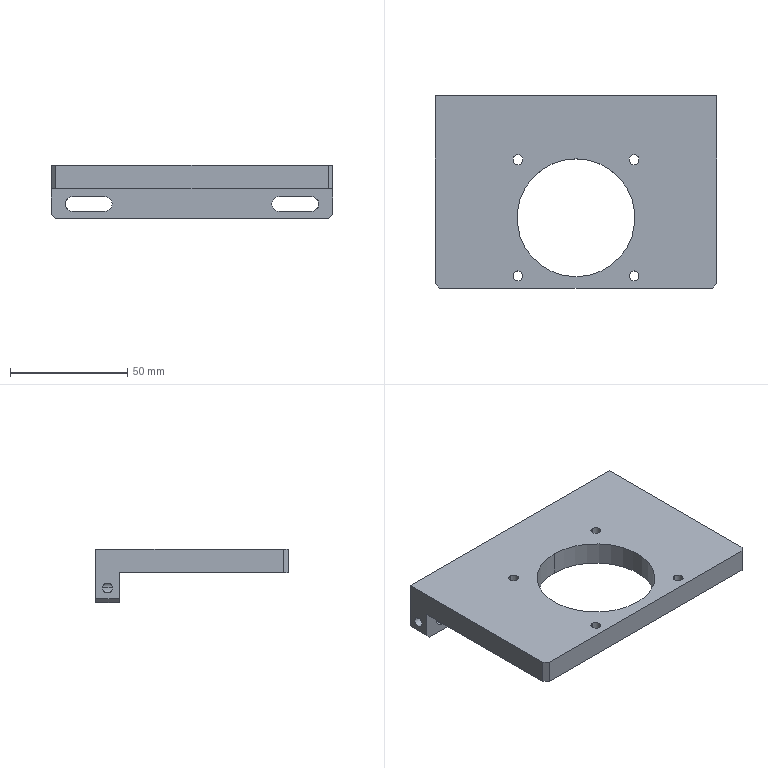NC program | NX | posted with a generic post | part box 120 x 82 x 22.8 mm
Lines 1 to 877 of 2242:
N10 G17 G21 G94 G90
(ZLEVEL_PROFILE_COPY_1 , TOOL : D4)
N12 T11 M6
N14 G54
N16 G17 G0 G90 X-42.486 Y6.25 B0. C0. S9500 M3
N18 G43 Z30. H11
N20 Z1.5
N22 G94 G1 X-51.114 Z1.048 F1000.
N24 X-51.591 Y6.018 Z1.02
N26 X-51.919 Y5.6 Z0.992
N28 X-52.03 Y5.084 Z0.964
N30 X-51.909 Y4.579 Z0.937
N32 X-51.582 Y4.175 Z0.91
N34 X-51.114 Y3.95 Z0.883
N36 X-36.886 Z0.137
N38 X-36.305 Y4.277 Z0.102
N40 X-35.993 Y4.866 Z0.067
N42 X-36.007 Y5.394 Z0.04
N44 X-36.327 Y5.945 Z0.006
N46 X-36.886 Y6.25 Z-0.027
N48 X-44. Z-0.4
N50 X-50.85 F1500.
N52 G3 X-52. Y5.1 R1.15
N54 X-50.85 Y3.95 R1.15
N56 G1 X-37.15
N58 G3 X-36. Y5.1 R1.15
N60 X-37.15 Y6.25 R1.15
N62 G1 X-44.
N64 X-45.713 Z-0.42
N66 X-47.425 Z-0.44
N68 X-49.138 Z-0.459
N70 X-50.85 Y6.233 Z-0.479
N72 X-51.18 Y6.18 Z-0.483
N74 X-51.343 Y6.112 Z-0.485
N76 X-51.518 Y6.004 Z-0.488
N78 X-51.652 Y5.902 Z-0.49
N80 X-51.734 Y5.793 Z-0.491
N82 X-51.906 Y5.487 Z-0.495
N84 X-51.952 Y5.337 Z-0.497
N86 X-51.976 Y5.035 Z-0.501
N88 X-51.95 Y4.838 Z-0.503
N90 X-51.85 Y4.575 Z-0.506
N92 X-51.726 Y4.393 Z-0.509
N94 X-51.513 Y4.191 Z-0.512
N96 X-51.335 Y4.084 Z-0.515
N98 X-51.2 Y4.028 Z-0.517
N100 X-51.131 Y4.003
N102 X-51.037 Y3.99 Z-0.519
N104 X-50.85 Y3.967 Z-0.521
N106 X-49.138 Y3.95 Z-0.541
N108 X-38.863 Z-0.659
N110 X-37.15 Y3.967 Z-0.679
N112 X-36.869 Y4.002 Z-0.683
N114 X-36.713 Y4.065 Z-0.684
N116 X-36.447 Y4.222 Z-0.688
N118 X-36.338 Y4.309 Z-0.69
N120 X-36.197 Y4.496 Z-0.693
N122 X-36.102 Y4.69 Z-0.695
N124 X-36.035 Y4.953 Z-0.698
N126 X-36.019 Y5.13 Z-0.7
N128 X-36.049 Y5.357 Z-0.703
N130 X-36.119 Y5.551 Z-0.705
N132 X-36.26 Y5.788 Z-0.709
N134 X-36.359 Y5.912 Z-0.711
N136 X-36.534 Y6.043 Z-0.713
N138 X-36.727 Y6.141 Z-0.716
N140 X-36.914 Y6.204 Z-0.718
N142 X-37.15 Y6.233 Z-0.721
N144 X-38.863 Y6.25 Z-0.741
N146 X-40.575 Z-0.76
N148 X-42.288 Z-0.78
N150 X-44. Z-0.8
N152 X-45.713 Z-0.82
N154 X-47.425 Z-0.84
N156 X-49.138 Z-0.859
N158 X-50.85 Y6.233 Z-0.879
N160 X-51.18 Y6.18 Z-0.883
N162 X-51.343 Y6.112 Z-0.885
N164 X-51.518 Y6.004 Z-0.888
N166 X-51.652 Y5.902 Z-0.89
N168 X-51.734 Y5.793 Z-0.891
N170 X-51.906 Y5.487 Z-0.895
N172 X-51.952 Y5.337 Z-0.897
N174 X-51.976 Y5.035 Z-0.901
N176 X-51.95 Y4.838 Z-0.903
N178 X-51.85 Y4.575 Z-0.906
N180 X-51.726 Y4.393 Z-0.909
N182 X-51.513 Y4.191 Z-0.912
N184 X-51.335 Y4.084 Z-0.915
N186 X-51.2 Y4.028 Z-0.917
N188 X-51.131 Y4.003
N190 X-51.037 Y3.99 Z-0.919
N192 X-50.85 Y3.967 Z-0.921
N194 X-49.138 Y3.95 Z-0.941
N196 X-38.863 Z-1.059
N198 X-37.15 Y3.967 Z-1.079
N200 X-36.869 Y4.002 Z-1.083
N202 X-36.713 Y4.065 Z-1.084
N204 X-36.447 Y4.222 Z-1.088
N206 X-36.338 Y4.309 Z-1.09
N208 X-36.197 Y4.496 Z-1.093
N210 X-36.102 Y4.69 Z-1.095
N212 X-36.035 Y4.953 Z-1.098
N214 X-36.019 Y5.13 Z-1.1
N216 X-36.049 Y5.357 Z-1.103
N218 X-36.119 Y5.551 Z-1.105
N220 X-36.26 Y5.788 Z-1.109
N222 X-36.359 Y5.912 Z-1.111
N224 X-36.534 Y6.043 Z-1.113
N226 X-36.727 Y6.141 Z-1.116
N228 X-36.914 Y6.204 Z-1.118
N230 X-37.15 Y6.233 Z-1.121
N232 X-38.863 Y6.25 Z-1.141
N234 X-40.575 Z-1.16
N236 X-42.288 Z-1.18
N238 X-44. Z-1.2
N240 X-45.713 Z-1.22
N242 X-47.425 Z-1.24
N244 X-49.138 Z-1.259
N246 X-50.85 Y6.233 Z-1.279
N248 X-51.18 Y6.18 Z-1.283
N250 X-51.343 Y6.112 Z-1.285
N252 X-51.518 Y6.004 Z-1.288
N254 X-51.652 Y5.902 Z-1.29
N256 X-51.734 Y5.793 Z-1.291
N258 X-51.906 Y5.487 Z-1.295
N260 X-51.952 Y5.337 Z-1.297
N262 X-51.976 Y5.035 Z-1.301
N264 X-51.95 Y4.838 Z-1.303
N266 X-51.85 Y4.575 Z-1.306
N268 X-51.726 Y4.393 Z-1.309
N270 X-51.513 Y4.191 Z-1.312
N272 X-51.335 Y4.084 Z-1.315
N274 X-51.2 Y4.028 Z-1.317
N276 X-51.131 Y4.003
N278 X-51.037 Y3.99 Z-1.319
N280 X-50.85 Y3.967 Z-1.321
N282 X-49.138 Y3.95 Z-1.341
N284 X-38.863 Z-1.459
N286 X-37.15 Y3.967 Z-1.479
N288 X-36.869 Y4.002 Z-1.483
N290 X-36.713 Y4.065 Z-1.484
N292 X-36.447 Y4.222 Z-1.488
N294 X-36.338 Y4.309 Z-1.49
N296 X-36.197 Y4.496 Z-1.493
N298 X-36.102 Y4.69 Z-1.495
N300 X-36.035 Y4.953 Z-1.498
N302 X-36.019 Y5.13 Z-1.5
N304 X-36.049 Y5.357 Z-1.503
N306 X-36.119 Y5.551 Z-1.505
N308 X-36.26 Y5.788 Z-1.509
N310 X-36.359 Y5.912 Z-1.511
N312 X-36.534 Y6.043 Z-1.513
N314 X-36.727 Y6.141 Z-1.516
N316 X-36.914 Y6.204 Z-1.518
N318 X-37.15 Y6.233 Z-1.521
N320 X-38.863 Y6.25 Z-1.541
N322 X-40.575 Z-1.56
N324 X-42.288 Z-1.58
N326 X-44. Z-1.6
N328 X-45.713 Z-1.62
N330 X-47.425 Z-1.64
N332 X-49.138 Z-1.659
N334 X-50.85 Y6.233 Z-1.679
N336 X-51.18 Y6.18 Z-1.683
N338 X-51.343 Y6.112 Z-1.685
N340 X-51.518 Y6.004 Z-1.688
N342 X-51.652 Y5.902 Z-1.69
N344 X-51.734 Y5.793 Z-1.691
N346 X-51.906 Y5.487 Z-1.695
N348 X-51.952 Y5.337 Z-1.697
N350 X-51.976 Y5.035 Z-1.701
N352 X-51.95 Y4.838 Z-1.703
N354 X-51.85 Y4.575 Z-1.706
N356 X-51.726 Y4.393 Z-1.709
N358 X-51.513 Y4.191 Z-1.712
N360 X-51.335 Y4.084 Z-1.715
N362 X-51.2 Y4.028 Z-1.717
N364 X-51.131 Y4.003
N366 X-51.037 Y3.99 Z-1.719
N368 X-50.85 Y3.967 Z-1.721
N370 X-49.138 Y3.95 Z-1.741
N372 X-38.863 Z-1.859
N374 X-37.15 Y3.967 Z-1.879
N376 X-36.869 Y4.002 Z-1.883
N378 X-36.713 Y4.065 Z-1.884
N380 X-36.447 Y4.222 Z-1.888
N382 X-36.338 Y4.309 Z-1.89
N384 X-36.197 Y4.496 Z-1.893
N386 X-36.102 Y4.69 Z-1.895
N388 X-36.035 Y4.953 Z-1.898
N390 X-36.019 Y5.13 Z-1.9
N392 X-36.049 Y5.357 Z-1.903
N394 X-36.119 Y5.551 Z-1.905
N396 X-36.26 Y5.788 Z-1.909
N398 X-36.359 Y5.912 Z-1.911
N400 X-36.534 Y6.043 Z-1.913
N402 X-36.727 Y6.141 Z-1.916
N404 X-36.914 Y6.204 Z-1.918
N406 X-37.15 Y6.233 Z-1.921
N408 X-38.863 Y6.25 Z-1.941
N410 X-40.575 Z-1.96
N412 X-42.288 Z-1.98
N414 X-44. Z-2.
N416 X-45.713 Z-2.02
N418 X-47.425 Z-2.04
N420 X-49.138 Z-2.059
N422 X-50.85 Y6.233 Z-2.079
N424 X-51.18 Y6.18 Z-2.083
N426 X-51.343 Y6.112 Z-2.085
N428 X-51.518 Y6.004 Z-2.088
N430 X-51.652 Y5.902 Z-2.09
N432 X-51.734 Y5.793 Z-2.091
N434 X-51.906 Y5.487 Z-2.095
N436 X-51.952 Y5.337 Z-2.097
N438 X-51.976 Y5.035 Z-2.101
N440 X-51.95 Y4.838 Z-2.103
N442 X-51.85 Y4.575 Z-2.106
N444 X-51.726 Y4.393 Z-2.109
N446 X-51.513 Y4.191 Z-2.112
N448 X-51.335 Y4.084 Z-2.115
N450 X-51.2 Y4.028 Z-2.117
N452 X-51.131 Y4.003
N454 X-51.037 Y3.99 Z-2.119
N456 X-50.85 Y3.967 Z-2.121
N458 X-49.138 Y3.95 Z-2.141
N460 X-38.863 Z-2.259
N462 X-37.15 Y3.967 Z-2.279
N464 X-36.869 Y4.002 Z-2.283
N466 X-36.713 Y4.065 Z-2.284
N468 X-36.447 Y4.222 Z-2.288
N470 X-36.338 Y4.309 Z-2.29
N472 X-36.197 Y4.496 Z-2.293
N474 X-36.102 Y4.69 Z-2.295
N476 X-36.035 Y4.953 Z-2.298
N478 X-36.019 Y5.13 Z-2.3
N480 X-36.049 Y5.357 Z-2.303
N482 X-36.119 Y5.551 Z-2.305
N484 X-36.26 Y5.788 Z-2.309
N486 X-36.359 Y5.912 Z-2.311
N488 X-36.534 Y6.043 Z-2.313
N490 X-36.727 Y6.141 Z-2.316
N492 X-36.914 Y6.204 Z-2.318
N494 X-37.15 Y6.233 Z-2.321
N496 X-38.863 Y6.25 Z-2.341
N498 X-40.575 Z-2.36
N500 X-42.288 Z-2.38
N502 X-44. Z-2.4
N504 X-45.713 Z-2.42
N506 X-47.425 Z-2.44
N508 X-49.138 Z-2.459
N510 X-50.85 Y6.233 Z-2.479
N512 X-51.18 Y6.18 Z-2.483
N514 X-51.343 Y6.112 Z-2.485
N516 X-51.518 Y6.004 Z-2.488
N518 X-51.652 Y5.902 Z-2.49
N520 X-51.734 Y5.793 Z-2.491
N522 X-51.906 Y5.487 Z-2.495
N524 X-51.952 Y5.337 Z-2.497
N526 X-51.976 Y5.035 Z-2.501
N528 X-51.95 Y4.838 Z-2.503
N530 X-51.85 Y4.575 Z-2.506
N532 X-51.726 Y4.393 Z-2.509
N534 X-51.513 Y4.191 Z-2.512
N536 X-51.335 Y4.084 Z-2.515
N538 X-51.2 Y4.028 Z-2.517
N540 X-51.131 Y4.003
N542 X-51.037 Y3.99 Z-2.519
N544 X-50.85 Y3.967 Z-2.521
N546 X-49.138 Y3.95 Z-2.541
N548 X-38.863 Z-2.659
N550 X-37.15 Y3.967 Z-2.679
N552 X-36.869 Y4.002 Z-2.683
N554 X-36.713 Y4.065 Z-2.684
N556 X-36.447 Y4.222 Z-2.688
N558 X-36.338 Y4.309 Z-2.69
N560 X-36.197 Y4.496 Z-2.693
N562 X-36.102 Y4.69 Z-2.695
N564 X-36.035 Y4.953 Z-2.698
N566 X-36.019 Y5.13 Z-2.7
N568 X-36.049 Y5.357 Z-2.703
N570 X-36.119 Y5.551 Z-2.705
N572 X-36.26 Y5.788 Z-2.709
N574 X-36.359 Y5.912 Z-2.711
N576 X-36.534 Y6.043 Z-2.713
N578 X-36.727 Y6.141 Z-2.716
N580 X-36.914 Y6.204 Z-2.718
N582 X-37.15 Y6.233 Z-2.721
N584 X-38.863 Y6.25 Z-2.741
N586 X-40.575 Z-2.76
N588 X-42.288 Z-2.78
N590 X-44. Z-2.8
N592 X-45.713 Z-2.82
N594 X-47.425 Z-2.84
N596 X-49.138 Z-2.859
N598 X-50.85 Y6.233 Z-2.879
N600 X-51.18 Y6.18 Z-2.883
N602 X-51.343 Y6.112 Z-2.885
N604 X-51.518 Y6.004 Z-2.888
N606 X-51.652 Y5.902 Z-2.89
N608 X-51.734 Y5.793 Z-2.891
N610 X-51.906 Y5.487 Z-2.895
N612 X-51.952 Y5.337 Z-2.897
N614 X-51.976 Y5.035 Z-2.901
N616 X-51.95 Y4.838 Z-2.903
N618 X-51.85 Y4.575 Z-2.906
N620 X-51.726 Y4.393 Z-2.909
N622 X-51.513 Y4.191 Z-2.912
N624 X-51.335 Y4.084 Z-2.915
N626 X-51.2 Y4.028 Z-2.917
N628 X-51.131 Y4.003
N630 X-51.037 Y3.99 Z-2.919
N632 X-50.85 Y3.967 Z-2.921
N634 X-49.138 Y3.95 Z-2.941
N636 X-38.863 Z-3.059
N638 X-37.15 Y3.967 Z-3.079
N640 X-36.869 Y4.002 Z-3.083
N642 X-36.713 Y4.065 Z-3.084
N644 X-36.447 Y4.222 Z-3.088
N646 X-36.338 Y4.309 Z-3.09
N648 X-36.197 Y4.496 Z-3.093
N650 X-36.102 Y4.69 Z-3.095
N652 X-36.035 Y4.953 Z-3.098
N654 X-36.019 Y5.13 Z-3.1
N656 X-36.049 Y5.357 Z-3.103
N658 X-36.119 Y5.551 Z-3.105
N660 X-36.26 Y5.788 Z-3.109
N662 X-36.359 Y5.912 Z-3.111
N664 X-36.534 Y6.043 Z-3.113
N666 X-36.727 Y6.141 Z-3.116
N668 X-36.914 Y6.204 Z-3.118
N670 X-37.15 Y6.233 Z-3.121
N672 X-38.863 Y6.25 Z-3.141
N674 X-40.575 Z-3.16
N676 X-42.288 Z-3.18
N678 X-44. Z-3.2
N680 X-45.713 Z-3.22
N682 X-47.425 Z-3.24
N684 X-49.138 Z-3.259
N686 X-50.85 Y6.233 Z-3.279
N688 X-51.18 Y6.18 Z-3.283
N690 X-51.343 Y6.112 Z-3.285
N692 X-51.518 Y6.004 Z-3.288
N694 X-51.652 Y5.902 Z-3.29
N696 X-51.734 Y5.793 Z-3.291
N698 X-51.906 Y5.487 Z-3.295
N700 X-51.952 Y5.337 Z-3.297
N702 X-51.976 Y5.035 Z-3.301
N704 X-51.95 Y4.838 Z-3.303
N706 X-51.85 Y4.575 Z-3.306
N708 X-51.726 Y4.393 Z-3.309
N710 X-51.513 Y4.191 Z-3.312
N712 X-51.335 Y4.084 Z-3.315
N714 X-51.2 Y4.028 Z-3.317
N716 X-51.131 Y4.003
N718 X-51.037 Y3.99 Z-3.319
N720 X-50.85 Y3.967 Z-3.321
N722 X-49.138 Y3.95 Z-3.341
N724 X-38.863 Z-3.459
N726 X-37.15 Y3.967 Z-3.479
N728 X-36.869 Y4.002 Z-3.483
N730 X-36.713 Y4.065 Z-3.484
N732 X-36.447 Y4.222 Z-3.488
N734 X-36.338 Y4.309 Z-3.49
N736 X-36.197 Y4.496 Z-3.493
N738 X-36.102 Y4.69 Z-3.495
N740 X-36.035 Y4.953 Z-3.498
N742 X-36.019 Y5.13 Z-3.5
N744 X-36.049 Y5.357 Z-3.503
N746 X-36.119 Y5.551 Z-3.505
N748 X-36.26 Y5.788 Z-3.509
N750 X-36.359 Y5.912 Z-3.511
N752 X-36.534 Y6.043 Z-3.513
N754 X-36.727 Y6.141 Z-3.516
N756 X-36.914 Y6.204 Z-3.518
N758 X-37.15 Y6.233 Z-3.521
N760 X-38.863 Y6.25 Z-3.541
N762 X-40.575 Z-3.56
N764 X-42.288 Z-3.58
N766 X-44. Z-3.6
N768 X-45.713 Z-3.62
N770 X-47.425 Z-3.64
N772 X-49.138 Z-3.659
N774 X-50.85 Y6.233 Z-3.679
N776 X-51.18 Y6.18 Z-3.683
N778 X-51.343 Y6.112 Z-3.685
N780 X-51.518 Y6.004 Z-3.688
N782 X-51.652 Y5.902 Z-3.69
N784 X-51.734 Y5.793 Z-3.691
N786 X-51.906 Y5.487 Z-3.695
N788 X-51.952 Y5.337 Z-3.697
N790 X-51.976 Y5.035 Z-3.701
N792 X-51.95 Y4.838 Z-3.703
N794 X-51.85 Y4.575 Z-3.706
N796 X-51.726 Y4.393 Z-3.709
N798 X-51.513 Y4.191 Z-3.712
N800 X-51.335 Y4.084 Z-3.715
N802 X-51.2 Y4.028 Z-3.717
N804 X-51.131 Y4.003
N806 X-51.037 Y3.99 Z-3.719
N808 X-50.85 Y3.967 Z-3.721
N810 X-49.138 Y3.95 Z-3.741
N812 X-38.863 Z-3.859
N814 X-37.15 Y3.967 Z-3.879
N816 X-36.869 Y4.002 Z-3.883
N818 X-36.713 Y4.065 Z-3.884
N820 X-36.447 Y4.222 Z-3.888
N822 X-36.338 Y4.309 Z-3.89
N824 X-36.197 Y4.496 Z-3.893
N826 X-36.102 Y4.69 Z-3.895
N828 X-36.035 Y4.953 Z-3.898
N830 X-36.019 Y5.13 Z-3.9
N832 X-36.049 Y5.357 Z-3.903
N834 X-36.119 Y5.551 Z-3.905
N836 X-36.26 Y5.788 Z-3.909
N838 X-36.359 Y5.912 Z-3.911
N840 X-36.534 Y6.043 Z-3.913
N842 X-36.727 Y6.141 Z-3.916
N844 X-36.914 Y6.204 Z-3.918
N846 X-37.15 Y6.233 Z-3.921
N848 X-38.863 Y6.25 Z-3.941
N850 X-40.575 Z-3.96
N852 X-42.288 Z-3.98
N854 X-44. Z-4.
N856 X-45.713 Z-4.02
N858 X-47.425 Z-4.04
N860 X-49.138 Z-4.059
N862 X-50.85 Y6.233 Z-4.079
N864 X-51.18 Y6.18 Z-4.083
N866 X-51.343 Y6.112 Z-4.085
N868 X-51.518 Y6.004 Z-4.088
N870 X-51.652 Y5.902 Z-4.09
N872 X-51.734 Y5.793 Z-4.091
N874 X-51.906 Y5.487 Z-4.095
N876 X-51.952 Y5.337 Z-4.097
N878 X-51.976 Y5.035 Z-4.101
N880 X-51.95 Y4.838 Z-4.103
N882 X-51.85 Y4.575 Z-4.106
N884 X-51.726 Y4.393 Z-4.109
N886 X-51.513 Y4.191 Z-4.112
N888 X-51.335 Y4.084 Z-4.115
N890 X-51.2 Y4.028 Z-4.117
N892 X-51.131 Y4.003
N894 X-51.037 Y3.99 Z-4.119
N896 X-50.85 Y3.967 Z-4.121
N898 X-49.138 Y3.95 Z-4.141
N900 X-38.863 Z-4.259
N902 X-37.15 Y3.967 Z-4.279
N904 X-36.869 Y4.002 Z-4.283
N906 X-36.713 Y4.065 Z-4.284
N908 X-36.447 Y4.222 Z-4.288
N910 X-36.338 Y4.309 Z-4.29
N912 X-36.197 Y4.496 Z-4.293
N914 X-36.102 Y4.69 Z-4.295
N916 X-36.035 Y4.953 Z-4.298
N918 X-36.019 Y5.13 Z-4.3
N920 X-36.049 Y5.357 Z-4.303
N922 X-36.119 Y5.551 Z-4.305
N924 X-36.26 Y5.788 Z-4.309
N926 X-36.359 Y5.912 Z-4.311
N928 X-36.534 Y6.043 Z-4.313
N930 X-36.727 Y6.141 Z-4.316
N932 X-36.914 Y6.204 Z-4.318
N934 X-37.15 Y6.233 Z-4.321
N936 X-38.863 Y6.25 Z-4.341
N938 X-40.575 Z-4.36
N940 X-42.288 Z-4.38
N942 X-44. Z-4.4
N944 X-45.713 Z-4.42
N946 X-47.425 Z-4.44
N948 X-49.138 Z-4.459
N950 X-50.85 Y6.233 Z-4.479
N952 X-51.18 Y6.18 Z-4.483
N954 X-51.343 Y6.112 Z-4.485
N956 X-51.518 Y6.004 Z-4.488
N958 X-51.652 Y5.902 Z-4.49
N960 X-51.734 Y5.793 Z-4.491
N962 X-51.906 Y5.487 Z-4.495
N964 X-51.952 Y5.337 Z-4.497
N966 X-51.976 Y5.035 Z-4.501
N968 X-51.95 Y4.838 Z-4.503
N970 X-51.85 Y4.575 Z-4.506
N972 X-51.726 Y4.393 Z-4.509
N974 X-51.513 Y4.191 Z-4.512
N976 X-51.335 Y4.084 Z-4.515
N978 X-51.2 Y4.028 Z-4.517
N980 X-51.131 Y4.003
N982 X-51.037 Y3.99 Z-4.519
N984 X-50.85 Y3.967 Z-4.521
N986 X-49.138 Y3.95 Z-4.541
N988 X-38.863 Z-4.659
N990 X-37.15 Y3.967 Z-4.679
N992 X-36.869 Y4.002 Z-4.683
N994 X-36.713 Y4.065 Z-4.684
N996 X-36.447 Y4.222 Z-4.688
N998 X-36.338 Y4.309 Z-4.69
N1000 X-36.197 Y4.496 Z-4.693
N1002 X-36.102 Y4.69 Z-4.695
N1004 X-36.035 Y4.953 Z-4.698
N1006 X-36.019 Y5.13 Z-4.7
N1008 X-36.049 Y5.357 Z-4.703
N1010 X-36.119 Y5.551 Z-4.705
N1012 X-36.26 Y5.788 Z-4.709
N1014 X-36.359 Y5.912 Z-4.711
N1016 X-36.534 Y6.043 Z-4.713
N1018 X-36.727 Y6.141 Z-4.716
N1020 X-36.914 Y6.204 Z-4.718
N1022 X-37.15 Y6.233 Z-4.721
N1024 X-38.863 Y6.25 Z-4.741
N1026 X-40.575 Z-4.76
N1028 X-42.288 Z-4.78
N1030 X-44. Z-4.8
N1032 X-45.713 Z-4.82
N1034 X-47.425 Z-4.84
N1036 X-49.138 Z-4.859
N1038 X-50.85 Y6.233 Z-4.879
N1040 X-51.18 Y6.18 Z-4.883
N1042 X-51.343 Y6.112 Z-4.885
N1044 X-51.518 Y6.004 Z-4.888
N1046 X-51.652 Y5.902 Z-4.89
N1048 X-51.734 Y5.793 Z-4.891
N1050 X-51.906 Y5.487 Z-4.895
N1052 X-51.952 Y5.337 Z-4.897
N1054 X-51.976 Y5.035 Z-4.901
N1056 X-51.95 Y4.838 Z-4.903
N1058 X-51.85 Y4.575 Z-4.906
N1060 X-51.726 Y4.393 Z-4.909
N1062 X-51.513 Y4.191 Z-4.912
N1064 X-51.335 Y4.084 Z-4.915
N1066 X-51.2 Y4.028 Z-4.917
N1068 X-51.131 Y4.003
N1070 X-51.037 Y3.99 Z-4.919
N1072 X-50.85 Y3.967 Z-4.921
N1074 X-49.138 Y3.95 Z-4.941
N1076 X-38.863 Z-5.059
N1078 X-37.15 Y3.967 Z-5.079
N1080 X-36.869 Y4.002 Z-5.083
N1082 X-36.713 Y4.065 Z-5.084
N1084 X-36.447 Y4.222 Z-5.088
N1086 X-36.338 Y4.309 Z-5.09
N1088 X-36.197 Y4.496 Z-5.093
N1090 X-36.102 Y4.69 Z-5.095
N1092 X-36.035 Y4.953 Z-5.098
N1094 X-36.019 Y5.13 Z-5.1
N1096 X-36.049 Y5.357 Z-5.103
N1098 X-36.119 Y5.551 Z-5.105
N1100 X-36.26 Y5.788 Z-5.109
N1102 X-36.359 Y5.912 Z-5.111
N1104 X-36.534 Y6.043 Z-5.113
N1106 X-36.727 Y6.141 Z-5.116
N1108 X-36.914 Y6.204 Z-5.118
N1110 X-37.15 Y6.233 Z-5.121
N1112 X-38.863 Y6.25 Z-5.141
N1114 X-40.575 Z-5.16
N1116 X-42.288 Z-5.18
N1118 X-44. Z-5.2
N1120 X-45.713 Z-5.22
N1122 X-47.425 Z-5.24
N1124 X-49.138 Z-5.259
N1126 X-50.85 Y6.233 Z-5.279
N1128 X-51.18 Y6.18 Z-5.283
N1130 X-51.343 Y6.112 Z-5.285
N1132 X-51.518 Y6.004 Z-5.288
N1134 X-51.652 Y5.902 Z-5.29
N1136 X-51.734 Y5.793 Z-5.291
N1138 X-51.906 Y5.487 Z-5.295
N1140 X-51.952 Y5.337 Z-5.297
N1142 X-51.976 Y5.035 Z-5.301
N1144 X-51.95 Y4.838 Z-5.303
N1146 X-51.85 Y4.575 Z-5.306
N1148 X-51.726 Y4.393 Z-5.309
N1150 X-51.513 Y4.191 Z-5.312
N1152 X-51.335 Y4.084 Z-5.315
N1154 X-51.2 Y4.028 Z-5.317
N1156 X-51.131 Y4.003
N1158 X-51.037 Y3.99 Z-5.319
N1160 X-50.85 Y3.967 Z-5.321
N1162 X-49.138 Y3.95 Z-5.341
N1164 X-38.863 Z-5.459
N1166 X-37.15 Y3.967 Z-5.479
N1168 X-36.869 Y4.002 Z-5.483
N1170 X-36.713 Y4.065 Z-5.484
N1172 X-36.447 Y4.222 Z-5.488
N1174 X-36.338 Y4.309 Z-5.49
N1176 X-36.197 Y4.496 Z-5.493
N1178 X-36.102 Y4.69 Z-5.495
N1180 X-36.035 Y4.953 Z-5.498
N1182 X-36.019 Y5.13 Z-5.5
N1184 X-36.049 Y5.357 Z-5.503
N1186 X-36.119 Y5.551 Z-5.505
N1188 X-36.26 Y5.788 Z-5.509
N1190 X-36.359 Y5.912 Z-5.511
N1192 X-36.534 Y6.043 Z-5.513
N1194 X-36.727 Y6.141 Z-5.516
N1196 X-36.914 Y6.204 Z-5.518
N1198 X-37.15 Y6.233 Z-5.521
N1200 X-38.863 Y6.25 Z-5.541
N1202 X-40.575 Z-5.56
N1204 X-42.288 Z-5.58
N1206 X-44. Z-5.6
N1208 X-45.713 Z-5.62
N1210 X-47.425 Z-5.64
N1212 X-49.138 Z-5.659
N1214 X-50.85 Y6.233 Z-5.679
N1216 X-51.18 Y6.18 Z-5.683
N1218 X-51.343 Y6.112 Z-5.685
N1220 X-51.518 Y6.004 Z-5.688
N1222 X-51.652 Y5.902 Z-5.69
N1224 X-51.734 Y5.793 Z-5.691
N1226 X-51.906 Y5.487 Z-5.695
N1228 X-51.952 Y5.337 Z-5.697
N1230 X-51.976 Y5.035 Z-5.701
N1232 X-51.95 Y4.838 Z-5.703
N1234 X-51.85 Y4.575 Z-5.706
N1236 X-51.726 Y4.393 Z-5.709
N1238 X-51.513 Y4.191 Z-5.712
N1240 X-51.335 Y4.084 Z-5.715
N1242 X-51.2 Y4.028 Z-5.717
N1244 X-51.131 Y4.003
N1246 X-51.037 Y3.99 Z-5.719
N1248 X-50.85 Y3.967 Z-5.721
N1250 X-49.138 Y3.95 Z-5.741
N1252 X-38.863 Z-5.859
N1254 X-37.15 Y3.967 Z-5.879
N1256 X-36.869 Y4.002 Z-5.883
N1258 X-36.713 Y4.065 Z-5.884
N1260 X-36.447 Y4.222 Z-5.888
N1262 X-36.338 Y4.309 Z-5.89
N1264 X-36.197 Y4.496 Z-5.893
N1266 X-36.102 Y4.69 Z-5.895
N1268 X-36.035 Y4.953 Z-5.898
N1270 X-36.019 Y5.13 Z-5.9
N1272 X-36.049 Y5.357 Z-5.903
N1274 X-36.119 Y5.551 Z-5.905
N1276 X-36.26 Y5.788 Z-5.909
N1278 X-36.359 Y5.912 Z-5.911
N1280 X-36.534 Y6.043 Z-5.913
N1282 X-36.727 Y6.141 Z-5.916
N1284 X-36.914 Y6.204 Z-5.918
N1286 X-37.15 Y6.233 Z-5.921
N1288 X-38.863 Y6.25 Z-5.941
N1290 X-40.575 Z-5.96
N1292 X-42.288 Z-5.98
N1294 X-44. Z-6.
N1296 X-45.713 Z-6.02
N1298 X-47.425 Z-6.04
N1300 X-49.138 Z-6.059
N1302 X-50.85 Y6.233 Z-6.079
N1304 X-51.18 Y6.18 Z-6.083
N1306 X-51.343 Y6.112 Z-6.085
N1308 X-51.518 Y6.004 Z-6.088
N1310 X-51.652 Y5.902 Z-6.09
N1312 X-51.734 Y5.793 Z-6.091
N1314 X-51.906 Y5.487 Z-6.095
N1316 X-51.952 Y5.337 Z-6.097
N1318 X-51.976 Y5.035 Z-6.101
N1320 X-51.95 Y4.838 Z-6.103
N1322 X-51.85 Y4.575 Z-6.106
N1324 X-51.726 Y4.393 Z-6.109
N1326 X-51.513 Y4.191 Z-6.112
N1328 X-51.335 Y4.084 Z-6.115
N1330 X-51.2 Y4.028 Z-6.117
N1332 X-51.131 Y4.003
N1334 X-51.037 Y3.99 Z-6.119
N1336 X-50.85 Y3.967 Z-6.121
N1338 X-49.138 Y3.95 Z-6.141
N1340 X-38.863 Z-6.259
N1342 X-37.15 Y3.967 Z-6.279
N1344 X-36.869 Y4.002 Z-6.283
N1346 X-36.713 Y4.065 Z-6.284
N1348 X-36.447 Y4.222 Z-6.288
N1350 X-36.338 Y4.309 Z-6.29
N1352 X-36.197 Y4.496 Z-6.293
N1354 X-36.102 Y4.69 Z-6.295
N1356 X-36.035 Y4.953 Z-6.298
N1358 X-36.019 Y5.13 Z-6.3
N1360 X-36.049 Y5.357 Z-6.303
N1362 X-36.119 Y5.551 Z-6.305
N1364 X-36.26 Y5.788 Z-6.309
N1366 X-36.359 Y5.912 Z-6.311
N1368 X-36.534 Y6.043 Z-6.313
N1370 X-36.727 Y6.141 Z-6.316
N1372 X-36.914 Y6.204 Z-6.318
N1374 X-37.15 Y6.233 Z-6.321
N1376 X-38.863 Y6.25 Z-6.341
N1378 X-40.575 Z-6.36
N1380 X-42.288 Z-6.38
N1382 X-44. Z-6.4
N1384 X-45.713 Z-6.42
N1386 X-47.425 Z-6.44
N1388 X-49.138 Z-6.459
N1390 X-50.85 Y6.233 Z-6.479
N1392 X-51.18 Y6.18 Z-6.483
N1394 X-51.343 Y6.112 Z-6.485
N1396 X-51.518 Y6.004 Z-6.488
N1398 X-51.652 Y5.902 Z-6.49
N1400 X-51.734 Y5.793 Z-6.491
N1402 X-51.906 Y5.487 Z-6.495
N1404 X-51.952 Y5.337 Z-6.497
N1406 X-51.976 Y5.035 Z-6.501
N1408 X-51.95 Y4.838 Z-6.503
N1410 X-51.85 Y4.575 Z-6.506
N1412 X-51.726 Y4.393 Z-6.509
N1414 X-51.513 Y4.191 Z-6.512
N1416 X-51.335 Y4.084 Z-6.515
N1418 X-51.2 Y4.028 Z-6.517
N1420 X-51.131 Y4.003
N1422 X-51.037 Y3.99 Z-6.519
N1424 X-50.85 Y3.967 Z-6.521
N1426 X-49.138 Y3.95 Z-6.541
N1428 X-38.863 Z-6.659
N1430 X-37.15 Y3.967 Z-6.679
N1432 X-36.869 Y4.002 Z-6.683
N1434 X-36.713 Y4.065 Z-6.684
N1436 X-36.447 Y4.222 Z-6.688
N1438 X-36.338 Y4.309 Z-6.69
N1440 X-36.197 Y4.496 Z-6.693
N1442 X-36.102 Y4.69 Z-6.695
N1444 X-36.035 Y4.953 Z-6.698
N1446 X-36.019 Y5.13 Z-6.7
N1448 X-36.049 Y5.357 Z-6.703
N1450 X-36.119 Y5.551 Z-6.705
N1452 X-36.26 Y5.788 Z-6.709
N1454 X-36.359 Y5.912 Z-6.711
N1456 X-36.534 Y6.043 Z-6.713
N1458 X-36.727 Y6.141 Z-6.716
N1460 X-36.914 Y6.204 Z-6.718
N1462 X-37.15 Y6.233 Z-6.721
N1464 X-38.863 Y6.25 Z-6.741
N1466 X-40.575 Z-6.76
N1468 X-42.288 Z-6.78
N1470 X-44. Z-6.8
N1472 X-45.713 Z-6.82
N1474 X-47.425 Z-6.84
N1476 X-49.138 Z-6.859
N1478 X-50.85 Y6.233 Z-6.879
N1480 X-51.18 Y6.18 Z-6.883
N1482 X-51.343 Y6.112 Z-6.885
N1484 X-51.518 Y6.004 Z-6.888
N1486 X-51.652 Y5.902 Z-6.89
N1488 X-51.734 Y5.793 Z-6.891
N1490 X-51.906 Y5.487 Z-6.895
N1492 X-51.952 Y5.337 Z-6.897
N1494 X-51.976 Y5.035 Z-6.901
N1496 X-51.95 Y4.838 Z-6.903
N1498 X-51.85 Y4.575 Z-6.906
N1500 X-51.726 Y4.393 Z-6.909
N1502 X-51.513 Y4.191 Z-6.912
N1504 X-51.335 Y4.084 Z-6.915
N1506 X-51.2 Y4.028 Z-6.917
N1508 X-51.131 Y4.003
N1510 X-51.037 Y3.99 Z-6.919
N1512 X-50.85 Y3.967 Z-6.921
N1514 X-49.138 Y3.95 Z-6.941
N1516 X-38.863 Z-7.059
N1518 X-37.15 Y3.967 Z-7.079
N1520 X-36.869 Y4.002 Z-7.083
N1522 X-36.713 Y4.065 Z-7.084
N1524 X-36.447 Y4.222 Z-7.088
N1526 X-36.338 Y4.309 Z-7.09
N1528 X-36.197 Y4.496 Z-7.093
N1530 X-36.102 Y4.69 Z-7.095
N1532 X-36.035 Y4.953 Z-7.098
N1534 X-36.019 Y5.13 Z-7.1
N1536 X-36.049 Y5.357 Z-7.103
N1538 X-36.119 Y5.551 Z-7.105
N1540 X-36.26 Y5.788 Z-7.109
N1542 X-36.359 Y5.912 Z-7.111
N1544 X-36.534 Y6.043 Z-7.113
N1546 X-36.727 Y6.141 Z-7.116
N1548 X-36.914 Y6.204 Z-7.118
N1550 X-37.15 Y6.233 Z-7.121
N1552 X-38.863 Y6.25 Z-7.141
N1554 X-40.575 Z-7.16
N1556 X-42.288 Z-7.18
N1558 X-44. Z-7.2
N1560 X-45.713 Z-7.22
N1562 X-47.425 Z-7.24
N1564 X-49.138 Z-7.259
N1566 X-50.85 Y6.233 Z-7.279
N1568 X-51.18 Y6.18 Z-7.283
N1570 X-51.343 Y6.112 Z-7.285
N1572 X-51.518 Y6.004 Z-7.288
N1574 X-51.652 Y5.902 Z-7.29
N1576 X-51.734 Y5.793 Z-7.291
N1578 X-51.906 Y5.487 Z-7.295
N1580 X-51.952 Y5.337 Z-7.297
N1582 X-51.976 Y5.035 Z-7.301
N1584 X-51.95 Y4.838 Z-7.303
N1586 X-51.85 Y4.575 Z-7.306
N1588 X-51.726 Y4.393 Z-7.309
N1590 X-51.513 Y4.191 Z-7.312
N1592 X-51.335 Y4.084 Z-7.315
N1594 X-51.2 Y4.028 Z-7.317
N1596 X-51.131 Y4.003
N1598 X-51.037 Y3.99 Z-7.319
N1600 X-50.85 Y3.967 Z-7.321
N1602 X-49.138 Y3.95 Z-7.341
N1604 X-38.863 Z-7.459
N1606 X-37.15 Y3.967 Z-7.479
N1608 X-36.869 Y4.002 Z-7.483
N1610 X-36.713 Y4.065 Z-7.484
N1612 X-36.447 Y4.222 Z-7.488
N1614 X-36.338 Y4.309 Z-7.49
N1616 X-36.197 Y4.496 Z-7.493
N1618 X-36.102 Y4.69 Z-7.495
N1620 X-36.035 Y4.953 Z-7.498
N1622 X-36.019 Y5.13 Z-7.5
N1624 X-36.049 Y5.357 Z-7.503
N1626 X-36.119 Y5.551 Z-7.505
N1628 X-36.26 Y5.788 Z-7.509
N1630 X-36.359 Y5.912 Z-7.511
N1632 X-36.534 Y6.043 Z-7.513
N1634 X-36.727 Y6.141 Z-7.516
N1636 X-36.914 Y6.204 Z-7.518
N1638 X-37.15 Y6.233 Z-7.521
N1640 X-38.863 Y6.25 Z-7.541
N1642 X-40.575 Z-7.56
N1644 X-42.288 Z-7.58
N1646 X-44. Z-7.6
N1648 X-45.713 Z-7.62
N1650 X-47.425 Z-7.64
N1652 X-49.138 Z-7.659
N1654 X-50.85 Y6.233 Z-7.679
N1656 X-51.18 Y6.18 Z-7.683
N1658 X-51.343 Y6.112 Z-7.685
N1660 X-51.518 Y6.004 Z-7.688
N1662 X-51.652 Y5.902 Z-7.69
N1664 X-51.734 Y5.793 Z-7.691
N1666 X-51.906 Y5.487 Z-7.695
N1668 X-51.952 Y5.337 Z-7.697
N1670 X-51.976 Y5.035 Z-7.701
N1672 X-51.95 Y4.838 Z-7.703
N1674 X-51.85 Y4.575 Z-7.706
N1676 X-51.726 Y4.393 Z-7.709
N1678 X-51.513 Y4.191 Z-7.712
N1680 X-51.335 Y4.084 Z-7.715
N1682 X-51.2 Y4.028 Z-7.717
N1684 X-51.131 Y4.003
N1686 X-51.037 Y3.99 Z-7.719
N1688 X-50.85 Y3.967 Z-7.721
N1690 X-49.138 Y3.95 Z-7.741
N1692 X-38.863 Z-7.859
N1694 X-37.15 Y3.967 Z-7.879
N1696 X-36.869 Y4.002 Z-7.883
N1698 X-36.713 Y4.065 Z-7.884
N1700 X-36.447 Y4.222 Z-7.888
N1702 X-36.338 Y4.309 Z-7.89
N1704 X-36.197 Y4.496 Z-7.893
N1706 X-36.102 Y4.69 Z-7.895
N1708 X-36.035 Y4.953 Z-7.898
N1710 X-36.019 Y5.13 Z-7.9
N1712 X-36.049 Y5.357 Z-7.903
N1714 X-36.119 Y5.551 Z-7.905
N1716 X-36.26 Y5.788 Z-7.909
N1718 X-36.359 Y5.912 Z-7.911
N1720 X-36.534 Y6.043 Z-7.913
N1722 X-36.727 Y6.141 Z-7.916
N1724 X-36.914 Y6.204 Z-7.918
N1726 X-37.15 Y6.233 Z-7.921
N1728 X-38.863 Y6.25 Z-7.941
N1730 X-40.575 Z-7.96
N1732 X-42.288 Z-7.98
N1734 X-44. Z-8.
N1736 X-45.713 Z-8.02
N1738 X-47.425 Z-8.04
N1740 X-49.138 Z-8.059
N1742 X-50.85 Y6.233 Z-8.079
N1744 X-51.18 Y6.18 Z-8.083
N1746 X-51.343 Y6.112 Z-8.085
N1748 X-51.518 Y6.004 Z-8.088
N1750 X-51.652 Y5.902 Z-8.09
N1752 X-51.734 Y5.793 Z-8.091